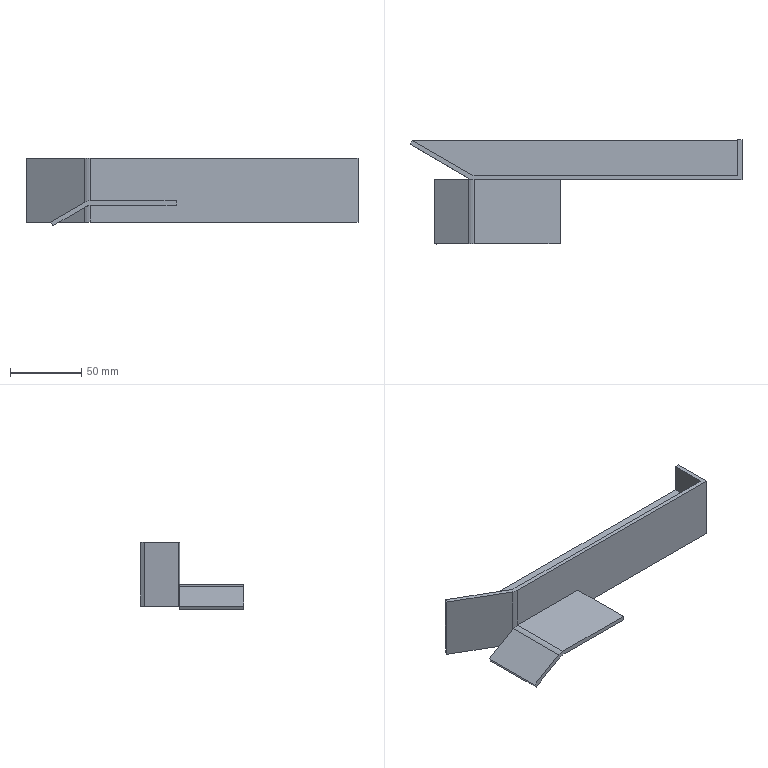Part | NX | features solid 2 | 1 solid | 28 faces | box 233.301 x 73 x 47.598 mm | volume 73994 mm3 | plane 23 | cylinder 5 | commonest cylinder face diameters 20 x3 16 x2
STEP:
#1=CARTESIAN_POINT('',(422.,443.,5.));
#2=VERTEX_POINT('',#1);
#3=CARTESIAN_POINT('',(238.483,443.,5.));
#4=VERTEX_POINT('',#3);
#5=CARTESIAN_POINT('',(422.,443.,5.));
#6=DIRECTION('',(1.,0.,0.));
#7=VECTOR('',#6,1000.);
#8=LINE('',#5,#7);
#9=EDGE_CURVE('',#2,#4,#8,.F.);
#10=ORIENTED_EDGE('',*,*,#9,.F.);
#11=CARTESIAN_POINT('',(422.,443.,-15.));
#12=VERTEX_POINT('',#11);
#13=CARTESIAN_POINT('',(422.,443.,-55.));
#14=DIRECTION('',(0.,0.,1.));
#15=VECTOR('',#14,1000.);
#16=LINE('',#13,#15);
#17=EDGE_CURVE('',#12,#2,#16,.T.);
#18=ORIENTED_EDGE('',*,*,#17,.F.);
#19=CARTESIAN_POINT('',(238.483,443.,-15.));
#20=VERTEX_POINT('',#19);
#21=CARTESIAN_POINT('',(265.,443.,-15.));
#22=DIRECTION('',(-1.,0.,0.));
#23=VECTOR('',#22,1000.);
#24=LINE('',#21,#23);
#25=EDGE_CURVE('',#12,#20,#24,.T.);
#26=ORIENTED_EDGE('',*,*,#25,.T.);
#27=CARTESIAN_POINT('',(238.483,443.,30.));
#28=DIRECTION('',(0.,0.,1.));
#29=VECTOR('',#28,1000.);
#30=LINE('',#27,#29);
#31=EDGE_CURVE('',#20,#4,#30,.T.);
#32=ORIENTED_EDGE('',*,*,#31,.T.);
#33=EDGE_LOOP('',(#10,#18,#26,#32));
#34=FACE_BOUND('',#33,.T.);
#35=CARTESIAN_POINT('',(265.,443.,30.));
#36=DIRECTION('',(0.,1.,0.));
#37=DIRECTION('',(0.,0.,1.));
#38=AXIS2_PLACEMENT_3D('',#35,#36,#37);
#39=PLANE('',#38);
#40=ADVANCED_FACE('',(#34),#39,.T.);
#41=CARTESIAN_POINT('',(422.,443.,10.));
#42=VERTEX_POINT('',#41);
#43=CARTESIAN_POINT('',(238.483,443.,10.));
#44=VERTEX_POINT('',#43);
#45=CARTESIAN_POINT('',(265.,443.,10.));
#46=DIRECTION('',(-1.,0.,0.));
#47=VECTOR('',#46,1000.);
#48=LINE('',#45,#47);
#49=EDGE_CURVE('',#42,#44,#48,.T.);
#50=ORIENTED_EDGE('',*,*,#49,.T.);
#51=CARTESIAN_POINT('',(238.483,443.,30.));
#52=VERTEX_POINT('',#51);
#53=CARTESIAN_POINT('',(238.483,443.,30.));
#54=DIRECTION('',(0.,0.,1.));
#55=VECTOR('',#54,1000.);
#56=LINE('',#53,#55);
#57=EDGE_CURVE('',#44,#52,#56,.T.);
#58=ORIENTED_EDGE('',*,*,#57,.T.);
#59=CARTESIAN_POINT('',(422.,443.,30.));
#60=VERTEX_POINT('',#59);
#61=CARTESIAN_POINT('',(265.,443.,30.));
#62=DIRECTION('',(1.,0.,0.));
#63=VECTOR('',#62,1000.);
#64=LINE('',#61,#63);
#65=EDGE_CURVE('',#60,#52,#64,.F.);
#66=ORIENTED_EDGE('',*,*,#65,.F.);
#67=CARTESIAN_POINT('',(422.,443.,-55.));
#68=DIRECTION('',(0.,0.,1.));
#69=VECTOR('',#68,1000.);
#70=LINE('',#67,#69);
#71=EDGE_CURVE('',#42,#60,#70,.T.);
#72=ORIENTED_EDGE('',*,*,#71,.F.);
#73=EDGE_LOOP('',(#50,#58,#66,#72));
#74=FACE_BOUND('',#73,.T.);
#75=CARTESIAN_POINT('',(265.,443.,30.));
#76=DIRECTION('',(0.,1.,0.));
#77=DIRECTION('',(0.,0.,1.));
#78=AXIS2_PLACEMENT_3D('',#75,#76,#77);
#79=PLANE('',#78);
#80=ADVANCED_FACE('',(#74),#79,.T.);
#81=CARTESIAN_POINT('',(233.483,444.34,5.));
#82=VERTEX_POINT('',#81);
#83=CARTESIAN_POINT('',(233.483,444.34,-15.));
#84=VERTEX_POINT('',#83);
#85=CARTESIAN_POINT('',(233.483,444.34,30.));
#86=DIRECTION('',(0.,0.,1.));
#87=VECTOR('',#86,1000.);
#88=LINE('',#85,#87);
#89=EDGE_CURVE('',#82,#84,#88,.F.);
#90=ORIENTED_EDGE('',*,*,#89,.F.);
#91=CARTESIAN_POINT('',(238.483,453.,5.));
#92=DIRECTION('',(0.,0.,-1.));
#93=DIRECTION('',(-1.,0.,0.));
#94=AXIS2_PLACEMENT_3D('',#91,#92,#93);
#95=CIRCLE('',#94,10.);
#96=EDGE_CURVE('',#82,#4,#95,.F.);
#97=ORIENTED_EDGE('',*,*,#96,.T.);
#98=ORIENTED_EDGE('',*,*,#31,.F.);
#99=CARTESIAN_POINT('',(238.483,453.,-15.));
#100=DIRECTION('',(0.,0.,1.));
#101=DIRECTION('',(1.,0.,0.));
#102=AXIS2_PLACEMENT_3D('',#99,#100,#101);
#103=CIRCLE('',#102,10.);
#104=EDGE_CURVE('',#84,#20,#103,.T.);
#105=ORIENTED_EDGE('',*,*,#104,.F.);
#106=EDGE_LOOP('',(#90,#97,#98,#105));
#107=FACE_BOUND('',#106,.T.);
#108=CARTESIAN_POINT('',(238.483,453.,30.));
#109=DIRECTION('',(0.,0.,1.));
#110=DIRECTION('',(1.,0.,0.));
#111=AXIS2_PLACEMENT_3D('',#108,#109,#110);
#112=CYLINDRICAL_SURFACE('',#111,10.);
#113=ADVANCED_FACE('',(#107),#112,.F.);
#114=ORIENTED_EDGE('',*,*,#57,.F.);
#115=CARTESIAN_POINT('',(233.483,444.34,10.));
#116=VERTEX_POINT('',#115);
#117=CARTESIAN_POINT('',(238.483,453.,10.));
#118=DIRECTION('',(0.,0.,-1.));
#119=DIRECTION('',(-1.,0.,0.));
#120=AXIS2_PLACEMENT_3D('',#117,#118,#119);
#121=CIRCLE('',#120,10.);
#122=EDGE_CURVE('',#44,#116,#121,.T.);
#123=ORIENTED_EDGE('',*,*,#122,.T.);
#124=CARTESIAN_POINT('',(233.483,444.34,30.));
#125=VERTEX_POINT('',#124);
#126=CARTESIAN_POINT('',(233.483,444.34,30.));
#127=DIRECTION('',(0.,0.,1.));
#128=VECTOR('',#127,1000.);
#129=LINE('',#126,#128);
#130=EDGE_CURVE('',#125,#116,#129,.F.);
#131=ORIENTED_EDGE('',*,*,#130,.F.);
#132=CARTESIAN_POINT('',(238.483,453.,30.));
#133=DIRECTION('',(0.,0.,1.));
#134=DIRECTION('',(1.,0.,0.));
#135=AXIS2_PLACEMENT_3D('',#132,#133,#134);
#136=CIRCLE('',#135,10.);
#137=EDGE_CURVE('',#52,#125,#136,.F.);
#138=ORIENTED_EDGE('',*,*,#137,.F.);
#139=EDGE_LOOP('',(#114,#123,#131,#138));
#140=FACE_BOUND('',#139,.T.);
#141=CARTESIAN_POINT('',(238.483,453.,30.));
#142=DIRECTION('',(0.,0.,1.));
#143=DIRECTION('',(1.,0.,0.));
#144=AXIS2_PLACEMENT_3D('',#141,#142,#143);
#145=CYLINDRICAL_SURFACE('',#144,10.);
#146=ADVANCED_FACE('',(#140),#145,.F.);
#147=ORIENTED_EDGE('',*,*,#17,.T.);
#148=CARTESIAN_POINT('',(422.,468.,5.));
#149=VERTEX_POINT('',#148);
#150=CARTESIAN_POINT('',(422.,468.,5.));
#151=DIRECTION('',(0.,1.,0.));
#152=VECTOR('',#151,1000.);
#153=LINE('',#150,#152);
#154=EDGE_CURVE('',#149,#2,#153,.F.);
#155=ORIENTED_EDGE('',*,*,#154,.F.);
#156=CARTESIAN_POINT('',(422.,468.,-15.));
#157=VERTEX_POINT('',#156);
#158=CARTESIAN_POINT('',(422.,468.,-50.));
#159=DIRECTION('',(0.,0.,-1.));
#160=VECTOR('',#159,1000.);
#161=LINE('',#158,#160);
#162=EDGE_CURVE('',#157,#149,#161,.F.);
#163=ORIENTED_EDGE('',*,*,#162,.F.);
#164=CARTESIAN_POINT('',(422.,460.,-15.));
#165=DIRECTION('',(0.,-1.,0.));
#166=VECTOR('',#165,1000.);
#167=LINE('',#164,#166);
#168=EDGE_CURVE('',#157,#12,#167,.T.);
#169=ORIENTED_EDGE('',*,*,#168,.T.);
#170=EDGE_LOOP('',(#147,#155,#163,#169));
#171=FACE_BOUND('',#170,.T.);
#172=CARTESIAN_POINT('',(422.,460.,-55.));
#173=DIRECTION('',(1.,0.,0.));
#174=DIRECTION('',(0.,0.,-1.));
#175=AXIS2_PLACEMENT_3D('',#172,#173,#174);
#176=PLANE('',#175);
#177=ADVANCED_FACE('',(#171),#176,.F.);
#178=CARTESIAN_POINT('',(422.,468.,10.));
#179=VERTEX_POINT('',#178);
#180=CARTESIAN_POINT('',(422.,468.,30.));
#181=VERTEX_POINT('',#180);
#182=CARTESIAN_POINT('',(422.,468.,-50.));
#183=DIRECTION('',(0.,0.,-1.));
#184=VECTOR('',#183,1000.);
#185=LINE('',#182,#184);
#186=EDGE_CURVE('',#179,#181,#185,.F.);
#187=ORIENTED_EDGE('',*,*,#186,.F.);
#188=CARTESIAN_POINT('',(422.,468.,10.));
#189=DIRECTION('',(0.,1.,0.));
#190=VECTOR('',#189,1000.);
#191=LINE('',#188,#190);
#192=EDGE_CURVE('',#179,#42,#191,.F.);
#193=ORIENTED_EDGE('',*,*,#192,.T.);
#194=ORIENTED_EDGE('',*,*,#71,.T.);
#195=CARTESIAN_POINT('',(422.,460.,30.));
#196=DIRECTION('',(0.,1.,0.));
#197=VECTOR('',#196,1000.);
#198=LINE('',#195,#197);
#199=EDGE_CURVE('',#181,#60,#198,.F.);
#200=ORIENTED_EDGE('',*,*,#199,.F.);
#201=EDGE_LOOP('',(#187,#193,#194,#200));
#202=FACE_BOUND('',#201,.T.);
#203=CARTESIAN_POINT('',(422.,460.,-55.));
#204=DIRECTION('',(1.,0.,0.));
#205=DIRECTION('',(0.,0.,-1.));
#206=AXIS2_PLACEMENT_3D('',#203,#204,#205);
#207=PLANE('',#206);
#208=ADVANCED_FACE('',(#202),#207,.F.);
#209=CARTESIAN_POINT('',(193.199,467.598,5.));
#210=VERTEX_POINT('',#209);
#211=CARTESIAN_POINT('',(193.199,467.598,-15.));
#212=VERTEX_POINT('',#211);
#213=CARTESIAN_POINT('',(193.199,467.598,30.));
#214=DIRECTION('',(0.,0.,-1.));
#215=VECTOR('',#214,1000.);
#216=LINE('',#213,#215);
#217=EDGE_CURVE('',#210,#212,#216,.T.);
#218=ORIENTED_EDGE('',*,*,#217,.F.);
#219=CARTESIAN_POINT('',(210.519,457.598,5.));
#220=DIRECTION('',(0.866,-0.5,0.));
#221=VECTOR('',#220,1000.);
#222=LINE('',#219,#221);
#223=EDGE_CURVE('',#210,#82,#222,.T.);
#224=ORIENTED_EDGE('',*,*,#223,.T.);
#225=ORIENTED_EDGE('',*,*,#89,.T.);
#226=CARTESIAN_POINT('',(250.34,434.608,-15.));
#227=DIRECTION('',(0.866,-0.5,0.));
#228=VECTOR('',#227,1000.);
#229=LINE('',#226,#228);
#230=EDGE_CURVE('',#212,#84,#229,.T.);
#231=ORIENTED_EDGE('',*,*,#230,.F.);
#232=EDGE_LOOP('',(#218,#224,#225,#231));
#233=FACE_BOUND('',#232,.T.);
#234=CARTESIAN_POINT('',(210.519,457.598,30.));
#235=DIRECTION('',(-0.5,-0.866,0.));
#236=DIRECTION('',(0.,0.,1.));
#237=AXIS2_PLACEMENT_3D('',#234,#235,#236);
#238=PLANE('',#237);
#239=ADVANCED_FACE('',(#233),#238,.F.);
#240=ORIENTED_EDGE('',*,*,#130,.T.);
#241=CARTESIAN_POINT('',(193.199,467.598,10.));
#242=VERTEX_POINT('',#241);
#243=CARTESIAN_POINT('',(364.626,368.625,10.));
#244=DIRECTION('',(-0.866,0.5,0.));
#245=VECTOR('',#244,1000.);
#246=LINE('',#243,#245);
#247=EDGE_CURVE('',#242,#116,#246,.F.);
#248=ORIENTED_EDGE('',*,*,#247,.F.);
#249=CARTESIAN_POINT('',(193.199,467.598,30.));
#250=VERTEX_POINT('',#249);
#251=CARTESIAN_POINT('',(193.199,467.598,30.));
#252=DIRECTION('',(0.,0.,-1.));
#253=VECTOR('',#252,1000.);
#254=LINE('',#251,#253);
#255=EDGE_CURVE('',#250,#242,#254,.T.);
#256=ORIENTED_EDGE('',*,*,#255,.F.);
#257=CARTESIAN_POINT('',(210.519,457.598,30.));
#258=DIRECTION('',(-0.866,0.5,0.));
#259=VECTOR('',#258,1000.);
#260=LINE('',#257,#259);
#261=EDGE_CURVE('',#250,#125,#260,.F.);
#262=ORIENTED_EDGE('',*,*,#261,.T.);
#263=EDGE_LOOP('',(#240,#248,#256,#262));
#264=FACE_BOUND('',#263,.T.);
#265=CARTESIAN_POINT('',(210.519,457.598,30.));
#266=DIRECTION('',(-0.5,-0.866,0.));
#267=DIRECTION('',(0.,0.,1.));
#268=AXIS2_PLACEMENT_3D('',#265,#266,#267);
#269=PLANE('',#268);
#270=ADVANCED_FACE('',(#264),#269,.F.);
#271=CARTESIAN_POINT('',(238.483,440.,-3.));
#272=VERTEX_POINT('',#271);
#273=CARTESIAN_POINT('',(237.144,440.,-3.09));
#274=VERTEX_POINT('',#273);
#275=CARTESIAN_POINT('',(238.483,440.,-13.));
#276=DIRECTION('',(0.,1.,0.));
#277=DIRECTION('',(1.,0.,0.));
#278=AXIS2_PLACEMENT_3D('',#275,#276,#277);
#279=CIRCLE('',#278,10.);
#280=EDGE_CURVE('',#272,#274,#279,.F.);
#281=ORIENTED_EDGE('',*,*,#280,.T.);
#282=CARTESIAN_POINT('',(237.144,440.,-15.));
#283=VERTEX_POINT('',#282);
#284=CARTESIAN_POINT('',(237.144,440.,-55.));
#285=DIRECTION('',(0.,0.,-1.));
#286=VECTOR('',#285,1000.);
#287=LINE('',#284,#286);
#288=EDGE_CURVE('',#274,#283,#287,.T.);
#289=ORIENTED_EDGE('',*,*,#288,.T.);
#290=CARTESIAN_POINT('',(425.,440.,-15.));
#291=VERTEX_POINT('',#290);
#292=CARTESIAN_POINT('',(265.,440.,-15.));
#293=DIRECTION('',(1.,0.,0.));
#294=VECTOR('',#293,1000.);
#295=LINE('',#292,#294);
#296=EDGE_CURVE('',#283,#291,#295,.T.);
#297=ORIENTED_EDGE('',*,*,#296,.T.);
#298=CARTESIAN_POINT('',(425.,440.,30.));
#299=VERTEX_POINT('',#298);
#300=CARTESIAN_POINT('',(425.,440.,-55.));
#301=DIRECTION('',(0.,0.,1.));
#302=VECTOR('',#301,1000.);
#303=LINE('',#300,#302);
#304=EDGE_CURVE('',#291,#299,#303,.T.);
#305=ORIENTED_EDGE('',*,*,#304,.T.);
#306=CARTESIAN_POINT('',(237.144,440.,30.));
#307=VERTEX_POINT('',#306);
#308=CARTESIAN_POINT('',(265.,440.,30.));
#309=DIRECTION('',(-1.,0.,0.));
#310=VECTOR('',#309,1000.);
#311=LINE('',#308,#310);
#312=EDGE_CURVE('',#307,#299,#311,.F.);
#313=ORIENTED_EDGE('',*,*,#312,.F.);
#314=CARTESIAN_POINT('',(237.144,440.,0.));
#315=VERTEX_POINT('',#314);
#316=CARTESIAN_POINT('',(237.144,440.,-55.));
#317=DIRECTION('',(0.,0.,-1.));
#318=VECTOR('',#317,1000.);
#319=LINE('',#316,#318);
#320=EDGE_CURVE('',#307,#315,#319,.T.);
#321=ORIENTED_EDGE('',*,*,#320,.T.);
#322=CARTESIAN_POINT('',(297.144,440.,0.));
#323=VERTEX_POINT('',#322);
#324=CARTESIAN_POINT('',(265.,440.,0.));
#325=DIRECTION('',(-1.,0.,0.));
#326=VECTOR('',#325,1000.);
#327=LINE('',#324,#326);
#328=EDGE_CURVE('',#315,#323,#327,.F.);
#329=ORIENTED_EDGE('',*,*,#328,.T.);
#330=CARTESIAN_POINT('',(297.144,440.,-3.));
#331=VERTEX_POINT('',#330);
#332=CARTESIAN_POINT('',(297.144,440.,-20.));
#333=DIRECTION('',(0.,0.,-1.));
#334=VECTOR('',#333,1000.);
#335=LINE('',#332,#334);
#336=EDGE_CURVE('',#331,#323,#335,.F.);
#337=ORIENTED_EDGE('',*,*,#336,.F.);
#338=CARTESIAN_POINT('',(265.,440.,-3.));
#339=DIRECTION('',(1.,0.,0.));
#340=VECTOR('',#339,1000.);
#341=LINE('',#338,#340);
#342=EDGE_CURVE('',#331,#272,#341,.F.);
#343=ORIENTED_EDGE('',*,*,#342,.T.);
#344=EDGE_LOOP('',(#281,#289,#297,#305,#313,#321,#329,#337,#343));
#345=FACE_BOUND('',#344,.T.);
#346=CARTESIAN_POINT('',(265.,440.,-55.));
#347=DIRECTION('',(0.,1.,0.));
#348=DIRECTION('',(0.,0.,1.));
#349=AXIS2_PLACEMENT_3D('',#346,#347,#348);
#350=PLANE('',#349);
#351=ADVANCED_FACE('',(#345),#350,.F.);
#352=ORIENTED_EDGE('',*,*,#296,.F.);
#353=CARTESIAN_POINT('',(233.144,441.072,-15.));
#354=VERTEX_POINT('',#353);
#355=CARTESIAN_POINT('',(237.144,448.,-15.));
#356=DIRECTION('',(0.,0.,1.));
#357=DIRECTION('',(1.,0.,0.));
#358=AXIS2_PLACEMENT_3D('',#355,#356,#357);
#359=CIRCLE('',#358,8.);
#360=EDGE_CURVE('',#283,#354,#359,.F.);
#361=ORIENTED_EDGE('',*,*,#360,.T.);
#362=CARTESIAN_POINT('',(191.699,465.,-15.));
#363=VERTEX_POINT('',#362);
#364=CARTESIAN_POINT('',(248.84,432.01,-15.));
#365=DIRECTION('',(0.866,-0.5,0.));
#366=VECTOR('',#365,1000.);
#367=LINE('',#364,#366);
#368=EDGE_CURVE('',#363,#354,#367,.T.);
#369=ORIENTED_EDGE('',*,*,#368,.F.);
#370=CARTESIAN_POINT('',(193.199,467.598,-15.));
#371=DIRECTION('',(0.5,0.866,0.));
#372=VECTOR('',#371,1000.);
#373=LINE('',#370,#372);
#374=EDGE_CURVE('',#363,#212,#373,.T.);
#375=ORIENTED_EDGE('',*,*,#374,.T.);
#376=ORIENTED_EDGE('',*,*,#230,.T.);
#377=ORIENTED_EDGE('',*,*,#104,.T.);
#378=ORIENTED_EDGE('',*,*,#25,.F.);
#379=ORIENTED_EDGE('',*,*,#168,.F.);
#380=CARTESIAN_POINT('',(425.,468.,-15.));
#381=VERTEX_POINT('',#380);
#382=CARTESIAN_POINT('',(265.,468.,-15.));
#383=DIRECTION('',(-1.,0.,0.));
#384=VECTOR('',#383,1000.);
#385=LINE('',#382,#384);
#386=EDGE_CURVE('',#157,#381,#385,.F.);
#387=ORIENTED_EDGE('',*,*,#386,.T.);
#388=CARTESIAN_POINT('',(425.,460.,-15.));
#389=DIRECTION('',(0.,-1.,0.));
#390=VECTOR('',#389,1000.);
#391=LINE('',#388,#390);
#392=EDGE_CURVE('',#381,#291,#391,.T.);
#393=ORIENTED_EDGE('',*,*,#392,.T.);
#394=EDGE_LOOP('',(#352,#361,#369,#375,#376,#377,#378,#379,#387,#393));
#395=FACE_BOUND('',#394,.T.);
#396=CARTESIAN_POINT('',(265.,460.,-15.));
#397=DIRECTION('',(0.,0.,1.));
#398=DIRECTION('',(0.,-1.,0.));
#399=AXIS2_PLACEMENT_3D('',#396,#397,#398);
#400=PLANE('',#399);
#401=ADVANCED_FACE('',(#395),#400,.F.);
#402=CARTESIAN_POINT('',(191.699,465.,30.));
#403=VERTEX_POINT('',#402);
#404=CARTESIAN_POINT('',(233.144,441.072,30.));
#405=VERTEX_POINT('',#404);
#406=CARTESIAN_POINT('',(209.019,455.,30.));
#407=DIRECTION('',(-0.866,0.5,0.));
#408=VECTOR('',#407,1000.);
#409=LINE('',#406,#408);
#410=EDGE_CURVE('',#403,#405,#409,.F.);
#411=ORIENTED_EDGE('',*,*,#410,.T.);
#412=CARTESIAN_POINT('',(237.144,448.,30.));
#413=DIRECTION('',(0.,0.,1.));
#414=DIRECTION('',(1.,0.,0.));
#415=AXIS2_PLACEMENT_3D('',#412,#413,#414);
#416=CIRCLE('',#415,8.);
#417=EDGE_CURVE('',#405,#307,#416,.T.);
#418=ORIENTED_EDGE('',*,*,#417,.T.);
#419=ORIENTED_EDGE('',*,*,#312,.T.);
#420=CARTESIAN_POINT('',(425.,468.,30.));
#421=VERTEX_POINT('',#420);
#422=CARTESIAN_POINT('',(425.,460.,30.));
#423=DIRECTION('',(0.,1.,0.));
#424=VECTOR('',#423,1000.);
#425=LINE('',#422,#424);
#426=EDGE_CURVE('',#421,#299,#425,.F.);
#427=ORIENTED_EDGE('',*,*,#426,.F.);
#428=CARTESIAN_POINT('',(315.,468.,30.));
#429=DIRECTION('',(1.,0.,0.));
#430=VECTOR('',#429,1000.);
#431=LINE('',#428,#430);
#432=EDGE_CURVE('',#181,#421,#431,.T.);
#433=ORIENTED_EDGE('',*,*,#432,.F.);
#434=ORIENTED_EDGE('',*,*,#199,.T.);
#435=ORIENTED_EDGE('',*,*,#65,.T.);
#436=ORIENTED_EDGE('',*,*,#137,.T.);
#437=ORIENTED_EDGE('',*,*,#261,.F.);
#438=CARTESIAN_POINT('',(207.859,492.99,30.));
#439=DIRECTION('',(-0.5,-0.866,0.));
#440=VECTOR('',#439,1000.);
#441=LINE('',#438,#440);
#442=EDGE_CURVE('',#403,#250,#441,.F.);
#443=ORIENTED_EDGE('',*,*,#442,.F.);
#444=EDGE_LOOP('',(#411,#418,#419,#427,#433,#434,#435,#436,#437,#443));
#445=FACE_BOUND('',#444,.T.);
#446=CARTESIAN_POINT('',(265.,460.,30.));
#447=DIRECTION('',(0.,0.,1.));
#448=DIRECTION('',(0.,-1.,0.));
#449=AXIS2_PLACEMENT_3D('',#446,#447,#448);
#450=PLANE('',#449);
#451=ADVANCED_FACE('',(#445),#450,.T.);
#452=ORIENTED_EDGE('',*,*,#426,.T.);
#453=ORIENTED_EDGE('',*,*,#304,.F.);
#454=ORIENTED_EDGE('',*,*,#392,.F.);
#455=CARTESIAN_POINT('',(425.,468.,-50.));
#456=DIRECTION('',(0.,0.,-1.));
#457=VECTOR('',#456,1000.);
#458=LINE('',#455,#457);
#459=EDGE_CURVE('',#381,#421,#458,.F.);
#460=ORIENTED_EDGE('',*,*,#459,.T.);
#461=EDGE_LOOP('',(#452,#453,#454,#460));
#462=FACE_BOUND('',#461,.T.);
#463=CARTESIAN_POINT('',(425.,460.,-55.));
#464=DIRECTION('',(1.,0.,0.));
#465=DIRECTION('',(0.,0.,-1.));
#466=AXIS2_PLACEMENT_3D('',#463,#464,#465);
#467=PLANE('',#466);
#468=ADVANCED_FACE('',(#462),#467,.T.);
#469=ORIENTED_EDGE('',*,*,#368,.T.);
#470=CARTESIAN_POINT('',(233.144,441.072,30.));
#471=DIRECTION('',(0.,0.,-1.));
#472=VECTOR('',#471,1000.);
#473=LINE('',#470,#472);
#474=EDGE_CURVE('',#354,#405,#473,.F.);
#475=ORIENTED_EDGE('',*,*,#474,.T.);
#476=ORIENTED_EDGE('',*,*,#410,.F.);
#477=CARTESIAN_POINT('',(191.699,465.,30.));
#478=DIRECTION('',(0.,0.,-1.));
#479=VECTOR('',#478,1000.);
#480=LINE('',#477,#479);
#481=EDGE_CURVE('',#403,#363,#480,.T.);
#482=ORIENTED_EDGE('',*,*,#481,.T.);
#483=EDGE_LOOP('',(#469,#475,#476,#482));
#484=FACE_BOUND('',#483,.T.);
#485=CARTESIAN_POINT('',(209.019,455.,30.));
#486=DIRECTION('',(-0.5,-0.866,0.));
#487=DIRECTION('',(0.,0.,1.));
#488=AXIS2_PLACEMENT_3D('',#485,#486,#487);
#489=PLANE('',#488);
#490=ADVANCED_FACE('',(#484),#489,.T.);
#491=ORIENTED_EDGE('',*,*,#417,.F.);
#492=ORIENTED_EDGE('',*,*,#474,.F.);
#493=ORIENTED_EDGE('',*,*,#360,.F.);
#494=ORIENTED_EDGE('',*,*,#288,.F.);
#495=CARTESIAN_POINT('',(237.144,440.,-55.));
#496=DIRECTION('',(0.,0.,-1.));
#497=VECTOR('',#496,1000.);
#498=LINE('',#495,#497);
#499=EDGE_CURVE('',#315,#274,#498,.T.);
#500=ORIENTED_EDGE('',*,*,#499,.F.);
#501=ORIENTED_EDGE('',*,*,#320,.F.);
#502=EDGE_LOOP('',(#491,#492,#493,#494,#500,#501));
#503=FACE_BOUND('',#502,.T.);
#504=CARTESIAN_POINT('',(237.144,448.,-55.));
#505=DIRECTION('',(0.,0.,1.));
#506=DIRECTION('',(1.,0.,0.));
#507=AXIS2_PLACEMENT_3D('',#504,#505,#506);
#508=CYLINDRICAL_SURFACE('',#507,8.);
#509=ADVANCED_FACE('',(#503),#508,.T.);
#510=CARTESIAN_POINT('',(297.144,395.,0.));
#511=VERTEX_POINT('',#510);
#512=CARTESIAN_POINT('',(297.144,395.,-3.));
#513=VERTEX_POINT('',#512);
#514=CARTESIAN_POINT('',(297.144,395.,-20.));
#515=DIRECTION('',(0.,0.,-1.));
#516=VECTOR('',#515,1000.);
#517=LINE('',#514,#516);
#518=EDGE_CURVE('',#511,#513,#517,.T.);
#519=ORIENTED_EDGE('',*,*,#518,.F.);
#520=CARTESIAN_POINT('',(237.144,395.,0.));
#521=VERTEX_POINT('',#520);
#522=CARTESIAN_POINT('',(265.,395.,0.));
#523=DIRECTION('',(1.,0.,0.));
#524=VECTOR('',#523,1000.);
#525=LINE('',#522,#524);
#526=EDGE_CURVE('',#521,#511,#525,.T.);
#527=ORIENTED_EDGE('',*,*,#526,.F.);
#528=CARTESIAN_POINT('',(233.144,395.,-1.072));
#529=VERTEX_POINT('',#528);
#530=CARTESIAN_POINT('',(237.144,395.,-8.));
#531=DIRECTION('',(0.,1.,0.));
#532=DIRECTION('',(1.,0.,0.));
#533=AXIS2_PLACEMENT_3D('',#530,#531,#532);
#534=CIRCLE('',#533,8.);
#535=EDGE_CURVE('',#521,#529,#534,.F.);
#536=ORIENTED_EDGE('',*,*,#535,.T.);
#537=CARTESIAN_POINT('',(209.019,395.,-15.));
#538=VERTEX_POINT('',#537);
#539=CARTESIAN_POINT('',(248.84,395.,7.99));
#540=DIRECTION('',(0.866,0.,0.5));
#541=VECTOR('',#540,1000.);
#542=LINE('',#539,#541);
#543=EDGE_CURVE('',#538,#529,#542,.T.);
#544=ORIENTED_EDGE('',*,*,#543,.F.);
#545=CARTESIAN_POINT('',(210.519,395.,-17.598));
#546=VERTEX_POINT('',#545);
#547=CARTESIAN_POINT('',(210.519,395.,-17.598));
#548=DIRECTION('',(0.5,0.,-0.866));
#549=VECTOR('',#548,1000.);
#550=LINE('',#547,#549);
#551=EDGE_CURVE('',#538,#546,#550,.T.);
#552=ORIENTED_EDGE('',*,*,#551,.T.);
#553=CARTESIAN_POINT('',(233.483,395.,-4.34));
#554=VERTEX_POINT('',#553);
#555=CARTESIAN_POINT('',(250.34,395.,5.392));
#556=DIRECTION('',(0.866,0.,0.5));
#557=VECTOR('',#556,1000.);
#558=LINE('',#555,#557);
#559=EDGE_CURVE('',#546,#554,#558,.T.);
#560=ORIENTED_EDGE('',*,*,#559,.T.);
#561=CARTESIAN_POINT('',(238.483,395.,-3.));
#562=VERTEX_POINT('',#561);
#563=CARTESIAN_POINT('',(238.483,395.,-13.));
#564=DIRECTION('',(0.,1.,0.));
#565=DIRECTION('',(1.,0.,0.));
#566=AXIS2_PLACEMENT_3D('',#563,#564,#565);
#567=CIRCLE('',#566,10.);
#568=EDGE_CURVE('',#554,#562,#567,.T.);
#569=ORIENTED_EDGE('',*,*,#568,.T.);
#570=CARTESIAN_POINT('',(265.,395.,-3.));
#571=DIRECTION('',(-1.,0.,0.));
#572=VECTOR('',#571,1000.);
#573=LINE('',#570,#572);
#574=EDGE_CURVE('',#513,#562,#573,.T.);
#575=ORIENTED_EDGE('',*,*,#574,.F.);
#576=EDGE_LOOP('',(#519,#527,#536,#544,#552,#560,#569,#575));
#577=FACE_BOUND('',#576,.T.);
#578=CARTESIAN_POINT('',(265.,395.,-20.));
#579=DIRECTION('',(0.,1.,0.));
#580=DIRECTION('',(0.,0.,1.));
#581=AXIS2_PLACEMENT_3D('',#578,#579,#580);
#582=PLANE('',#581);
#583=ADVANCED_FACE('',(#577),#582,.F.);
#584=CARTESIAN_POINT('',(297.144,355.,0.));
#585=DIRECTION('',(0.,-1.,0.));
#586=VECTOR('',#585,1000.);
#587=LINE('',#584,#586);
#588=EDGE_CURVE('',#323,#511,#587,.T.);
#589=ORIENTED_EDGE('',*,*,#588,.F.);
#590=ORIENTED_EDGE('',*,*,#328,.F.);
#591=CARTESIAN_POINT('',(237.144,355.,0.));
#592=DIRECTION('',(0.,-1.,0.));
#593=VECTOR('',#592,1000.);
#594=LINE('',#591,#593);
#595=EDGE_CURVE('',#315,#521,#594,.T.);
#596=ORIENTED_EDGE('',*,*,#595,.T.);
#597=ORIENTED_EDGE('',*,*,#526,.T.);
#598=EDGE_LOOP('',(#589,#590,#596,#597));
#599=FACE_BOUND('',#598,.T.);
#600=CARTESIAN_POINT('',(265.,355.,0.));
#601=DIRECTION('',(0.,0.,-1.));
#602=DIRECTION('',(0.,1.,0.));
#603=AXIS2_PLACEMENT_3D('',#600,#601,#602);
#604=PLANE('',#603);
#605=ADVANCED_FACE('',(#599),#604,.F.);
#606=ORIENTED_EDGE('',*,*,#499,.T.);
#607=CARTESIAN_POINT('',(233.483,440.,-4.34));
#608=VERTEX_POINT('',#607);
#609=CARTESIAN_POINT('',(238.483,440.,-13.));
#610=DIRECTION('',(0.,1.,0.));
#611=DIRECTION('',(1.,0.,0.));
#612=AXIS2_PLACEMENT_3D('',#609,#610,#611);
#613=CIRCLE('',#612,10.);
#614=EDGE_CURVE('',#274,#608,#613,.F.);
#615=ORIENTED_EDGE('',*,*,#614,.T.);
#616=CARTESIAN_POINT('',(210.519,440.,-17.598));
#617=VERTEX_POINT('',#616);
#618=CARTESIAN_POINT('',(210.519,440.,-17.598));
#619=DIRECTION('',(-0.866,0.,-0.5));
#620=VECTOR('',#619,1000.);
#621=LINE('',#618,#620);
#622=EDGE_CURVE('',#617,#608,#621,.F.);
#623=ORIENTED_EDGE('',*,*,#622,.F.);
#624=CARTESIAN_POINT('',(209.019,440.,-15.));
#625=VERTEX_POINT('',#624);
#626=CARTESIAN_POINT('',(225.179,440.,-42.99));
#627=DIRECTION('',(-0.5,0.,0.866));
#628=VECTOR('',#627,1000.);
#629=LINE('',#626,#628);
#630=EDGE_CURVE('',#625,#617,#629,.F.);
#631=ORIENTED_EDGE('',*,*,#630,.F.);
#632=CARTESIAN_POINT('',(233.144,440.,-1.072));
#633=VERTEX_POINT('',#632);
#634=CARTESIAN_POINT('',(209.019,440.,-15.));
#635=DIRECTION('',(-0.866,0.,-0.5));
#636=VECTOR('',#635,1000.);
#637=LINE('',#634,#636);
#638=EDGE_CURVE('',#625,#633,#637,.F.);
#639=ORIENTED_EDGE('',*,*,#638,.T.);
#640=CARTESIAN_POINT('',(237.144,440.,-8.));
#641=DIRECTION('',(0.,1.,0.));
#642=DIRECTION('',(1.,0.,0.));
#643=AXIS2_PLACEMENT_3D('',#640,#641,#642);
#644=CIRCLE('',#643,8.);
#645=EDGE_CURVE('',#633,#315,#644,.T.);
#646=ORIENTED_EDGE('',*,*,#645,.T.);
#647=EDGE_LOOP('',(#606,#615,#623,#631,#639,#646));
#648=FACE_BOUND('',#647,.T.);
#649=CARTESIAN_POINT('',(265.,440.,-20.));
#650=DIRECTION('',(0.,1.,0.));
#651=DIRECTION('',(0.,0.,1.));
#652=AXIS2_PLACEMENT_3D('',#649,#650,#651);
#653=PLANE('',#652);
#654=ADVANCED_FACE('',(#648),#653,.T.);
#655=ORIENTED_EDGE('',*,*,#574,.T.);
#656=CARTESIAN_POINT('',(238.483,440.,-3.));
#657=DIRECTION('',(0.,1.,0.));
#658=VECTOR('',#657,1000.);
#659=LINE('',#656,#658);
#660=EDGE_CURVE('',#562,#272,#659,.T.);
#661=ORIENTED_EDGE('',*,*,#660,.T.);
#662=ORIENTED_EDGE('',*,*,#342,.F.);
#663=CARTESIAN_POINT('',(297.144,395.,-3.));
#664=DIRECTION('',(0.,1.,0.));
#665=VECTOR('',#664,1000.);
#666=LINE('',#663,#665);
#667=EDGE_CURVE('',#513,#331,#666,.T.);
#668=ORIENTED_EDGE('',*,*,#667,.F.);
#669=EDGE_LOOP('',(#655,#661,#662,#668));
#670=FACE_BOUND('',#669,.T.);
#671=CARTESIAN_POINT('',(265.,440.,-3.));
#672=DIRECTION('',(0.,0.,-1.));
#673=DIRECTION('',(0.,1.,0.));
#674=AXIS2_PLACEMENT_3D('',#671,#672,#673);
#675=PLANE('',#674);
#676=ADVANCED_FACE('',(#670),#675,.T.);
#677=ORIENTED_EDGE('',*,*,#551,.F.);
#678=CARTESIAN_POINT('',(209.019,440.,-15.));
#679=DIRECTION('',(0.,1.,0.));
#680=VECTOR('',#679,1000.);
#681=LINE('',#678,#680);
#682=EDGE_CURVE('',#625,#538,#681,.F.);
#683=ORIENTED_EDGE('',*,*,#682,.F.);
#684=ORIENTED_EDGE('',*,*,#630,.T.);
#685=CARTESIAN_POINT('',(210.519,440.,-17.598));
#686=DIRECTION('',(0.,-1.,0.));
#687=VECTOR('',#686,1000.);
#688=LINE('',#685,#687);
#689=EDGE_CURVE('',#617,#546,#688,.T.);
#690=ORIENTED_EDGE('',*,*,#689,.T.);
#691=EDGE_LOOP('',(#677,#683,#684,#690));
#692=FACE_BOUND('',#691,.T.);
#693=CARTESIAN_POINT('',(210.519,440.,-17.598));
#694=DIRECTION('',(-0.866,0.,-0.5));
#695=DIRECTION('',(0.,-1.,0.));
#696=AXIS2_PLACEMENT_3D('',#693,#694,#695);
#697=PLANE('',#696);
#698=ADVANCED_FACE('',(#692),#697,.T.);
#699=ORIENTED_EDGE('',*,*,#622,.T.);
#700=CARTESIAN_POINT('',(233.483,440.,-4.34));
#701=DIRECTION('',(0.,1.,0.));
#702=VECTOR('',#701,1000.);
#703=LINE('',#700,#702);
#704=EDGE_CURVE('',#608,#554,#703,.F.);
#705=ORIENTED_EDGE('',*,*,#704,.T.);
#706=ORIENTED_EDGE('',*,*,#559,.F.);
#707=ORIENTED_EDGE('',*,*,#689,.F.);
#708=EDGE_LOOP('',(#699,#705,#706,#707));
#709=FACE_BOUND('',#708,.T.);
#710=CARTESIAN_POINT('',(210.519,440.,-17.598));
#711=DIRECTION('',(-0.5,0.,0.866));
#712=DIRECTION('',(0.,1.,0.));
#713=AXIS2_PLACEMENT_3D('',#710,#711,#712);
#714=PLANE('',#713);
#715=ADVANCED_FACE('',(#709),#714,.F.);
#716=ORIENTED_EDGE('',*,*,#543,.T.);
#717=CARTESIAN_POINT('',(233.144,440.,-1.072));
#718=DIRECTION('',(0.,-1.,0.));
#719=VECTOR('',#718,1000.);
#720=LINE('',#717,#719);
#721=EDGE_CURVE('',#529,#633,#720,.F.);
#722=ORIENTED_EDGE('',*,*,#721,.T.);
#723=ORIENTED_EDGE('',*,*,#638,.F.);
#724=ORIENTED_EDGE('',*,*,#682,.T.);
#725=EDGE_LOOP('',(#716,#722,#723,#724));
#726=FACE_BOUND('',#725,.T.);
#727=CARTESIAN_POINT('',(209.019,440.,-15.));
#728=DIRECTION('',(-0.5,0.,0.866));
#729=DIRECTION('',(0.,1.,0.));
#730=AXIS2_PLACEMENT_3D('',#727,#728,#729);
#731=PLANE('',#730);
#732=ADVANCED_FACE('',(#726),#731,.T.);
#733=ORIENTED_EDGE('',*,*,#568,.F.);
#734=ORIENTED_EDGE('',*,*,#704,.F.);
#735=ORIENTED_EDGE('',*,*,#614,.F.);
#736=ORIENTED_EDGE('',*,*,#280,.F.);
#737=ORIENTED_EDGE('',*,*,#660,.F.);
#738=EDGE_LOOP('',(#733,#734,#735,#736,#737));
#739=FACE_BOUND('',#738,.T.);
#740=CARTESIAN_POINT('',(238.483,440.,-13.));
#741=DIRECTION('',(0.,1.,0.));
#742=DIRECTION('',(1.,0.,0.));
#743=AXIS2_PLACEMENT_3D('',#740,#741,#742);
#744=CYLINDRICAL_SURFACE('',#743,10.);
#745=ADVANCED_FACE('',(#739),#744,.F.);
#746=ORIENTED_EDGE('',*,*,#645,.F.);
#747=ORIENTED_EDGE('',*,*,#721,.F.);
#748=ORIENTED_EDGE('',*,*,#535,.F.);
#749=ORIENTED_EDGE('',*,*,#595,.F.);
#750=EDGE_LOOP('',(#746,#747,#748,#749));
#751=FACE_BOUND('',#750,.T.);
#752=CARTESIAN_POINT('',(237.144,355.,-8.));
#753=DIRECTION('',(0.,1.,0.));
#754=DIRECTION('',(1.,0.,0.));
#755=AXIS2_PLACEMENT_3D('',#752,#753,#754);
#756=CYLINDRICAL_SURFACE('',#755,8.);
#757=ADVANCED_FACE('',(#751),#756,.T.);
#758=ORIENTED_EDGE('',*,*,#667,.T.);
#759=ORIENTED_EDGE('',*,*,#336,.T.);
#760=ORIENTED_EDGE('',*,*,#588,.T.);
#761=ORIENTED_EDGE('',*,*,#518,.T.);
#762=EDGE_LOOP('',(#758,#759,#760,#761));
#763=FACE_BOUND('',#762,.T.);
#764=CARTESIAN_POINT('',(297.144,395.,-3.));
#765=DIRECTION('',(1.,0.,0.));
#766=DIRECTION('',(0.,0.,-1.));
#767=AXIS2_PLACEMENT_3D('',#764,#765,#766);
#768=PLANE('',#767);
#769=ADVANCED_FACE('',(#763),#768,.T.);
#770=ORIENTED_EDGE('',*,*,#96,.F.);
#771=ORIENTED_EDGE('',*,*,#223,.F.);
#772=CARTESIAN_POINT('',(193.431,468.,5.));
#773=VERTEX_POINT('',#772);
#774=CARTESIAN_POINT('',(250.573,566.973,5.));
#775=DIRECTION('',(0.5,0.866,0.));
#776=VECTOR('',#775,1000.);
#777=LINE('',#774,#776);
#778=EDGE_CURVE('',#210,#773,#777,.T.);
#779=ORIENTED_EDGE('',*,*,#778,.T.);
#780=CARTESIAN_POINT('',(422.,468.,5.));
#781=DIRECTION('',(-1.,0.,0.));
#782=VECTOR('',#781,1000.);
#783=LINE('',#780,#782);
#784=EDGE_CURVE('',#149,#773,#783,.T.);
#785=ORIENTED_EDGE('',*,*,#784,.F.);
#786=ORIENTED_EDGE('',*,*,#154,.T.);
#787=ORIENTED_EDGE('',*,*,#9,.T.);
#788=EDGE_LOOP('',(#770,#771,#779,#785,#786,#787));
#789=FACE_BOUND('',#788,.T.);
#790=CARTESIAN_POINT('',(422.,468.,5.));
#791=DIRECTION('',(0.,0.,-1.));
#792=DIRECTION('',(-1.,0.,0.));
#793=AXIS2_PLACEMENT_3D('',#790,#791,#792);
#794=PLANE('',#793);
#795=ADVANCED_FACE('',(#789),#794,.T.);
#796=ORIENTED_EDGE('',*,*,#122,.F.);
#797=ORIENTED_EDGE('',*,*,#49,.F.);
#798=ORIENTED_EDGE('',*,*,#192,.F.);
#799=CARTESIAN_POINT('',(193.431,468.,10.));
#800=VERTEX_POINT('',#799);
#801=CARTESIAN_POINT('',(422.,468.,10.));
#802=DIRECTION('',(-1.,0.,0.));
#803=VECTOR('',#802,1000.);
#804=LINE('',#801,#803);
#805=EDGE_CURVE('',#179,#800,#804,.T.);
#806=ORIENTED_EDGE('',*,*,#805,.T.);
#807=CARTESIAN_POINT('',(250.573,566.973,10.));
#808=DIRECTION('',(0.5,0.866,0.));
#809=VECTOR('',#808,1000.);
#810=LINE('',#807,#809);
#811=EDGE_CURVE('',#800,#242,#810,.F.);
#812=ORIENTED_EDGE('',*,*,#811,.T.);
#813=ORIENTED_EDGE('',*,*,#247,.T.);
#814=EDGE_LOOP('',(#796,#797,#798,#806,#812,#813));
#815=FACE_BOUND('',#814,.T.);
#816=CARTESIAN_POINT('',(422.,468.,10.));
#817=DIRECTION('',(0.,0.,-1.));
#818=DIRECTION('',(-1.,0.,0.));
#819=AXIS2_PLACEMENT_3D('',#816,#817,#818);
#820=PLANE('',#819);
#821=ADVANCED_FACE('',(#815),#820,.F.);
#822=CARTESIAN_POINT('',(193.431,468.,10.));
#823=DIRECTION('',(0.,0.,1.));
#824=VECTOR('',#823,1000.);
#825=LINE('',#822,#824);
#826=EDGE_CURVE('',#800,#773,#825,.F.);
#827=ORIENTED_EDGE('',*,*,#826,.F.);
#828=ORIENTED_EDGE('',*,*,#805,.F.);
#829=ORIENTED_EDGE('',*,*,#186,.T.);
#830=ORIENTED_EDGE('',*,*,#432,.T.);
#831=ORIENTED_EDGE('',*,*,#459,.F.);
#832=ORIENTED_EDGE('',*,*,#386,.F.);
#833=ORIENTED_EDGE('',*,*,#162,.T.);
#834=ORIENTED_EDGE('',*,*,#784,.T.);
#835=EDGE_LOOP('',(#827,#828,#829,#830,#831,#832,#833,#834));
#836=FACE_BOUND('',#835,.T.);
#837=CARTESIAN_POINT('',(422.,468.,10.));
#838=DIRECTION('',(0.,1.,0.));
#839=DIRECTION('',(0.,0.,1.));
#840=AXIS2_PLACEMENT_3D('',#837,#838,#839);
#841=PLANE('',#840);
#842=ADVANCED_FACE('',(#836),#841,.T.);
#843=ORIENTED_EDGE('',*,*,#778,.F.);
#844=ORIENTED_EDGE('',*,*,#217,.T.);
#845=ORIENTED_EDGE('',*,*,#374,.F.);
#846=ORIENTED_EDGE('',*,*,#481,.F.);
#847=ORIENTED_EDGE('',*,*,#442,.T.);
#848=ORIENTED_EDGE('',*,*,#255,.T.);
#849=ORIENTED_EDGE('',*,*,#811,.F.);
#850=ORIENTED_EDGE('',*,*,#826,.T.);
#851=EDGE_LOOP('',(#843,#844,#845,#846,#847,#848,#849,#850));
#852=FACE_BOUND('',#851,.T.);
#853=CARTESIAN_POINT('',(193.199,467.598,30.));
#854=DIRECTION('',(-0.866,0.5,0.));
#855=DIRECTION('',(0.,0.,-1.));
#856=AXIS2_PLACEMENT_3D('',#853,#854,#855);
#857=PLANE('',#856);
#858=ADVANCED_FACE('',(#852),#857,.T.);
#859=CLOSED_SHELL('',(#40,#80,#113,#146,#177,#208,#239,#270,#351,#401,#451,#468,#490,#509,#583,#605,#654,#676,#698,#715,#732,#745,#757,#769,#795,#821,#842,#858));
#860=MANIFOLD_SOLID_BREP('',#859);
#861=(LENGTH_UNIT()NAMED_UNIT(*)SI_UNIT(.MILLI.,.METRE.));
#862=UNCERTAINTY_MEASURE_WITH_UNIT(LENGTH_MEASURE(0.00001),#861,'','');
#863=(NAMED_UNIT(*)PLANE_ANGLE_UNIT()SI_UNIT($,.RADIAN.));
#864=(NAMED_UNIT(*)SI_UNIT($,.STERADIAN.)SOLID_ANGLE_UNIT());
#865=(GEOMETRIC_REPRESENTATION_CONTEXT(3)GLOBAL_UNCERTAINTY_ASSIGNED_CONTEXT((#862))GLOBAL_UNIT_ASSIGNED_CONTEXT((#861,#863,#864))REPRESENTATION_CONTEXT('',''));
#866=ADVANCED_BREP_SHAPE_REPRESENTATION('',(#860),#865);